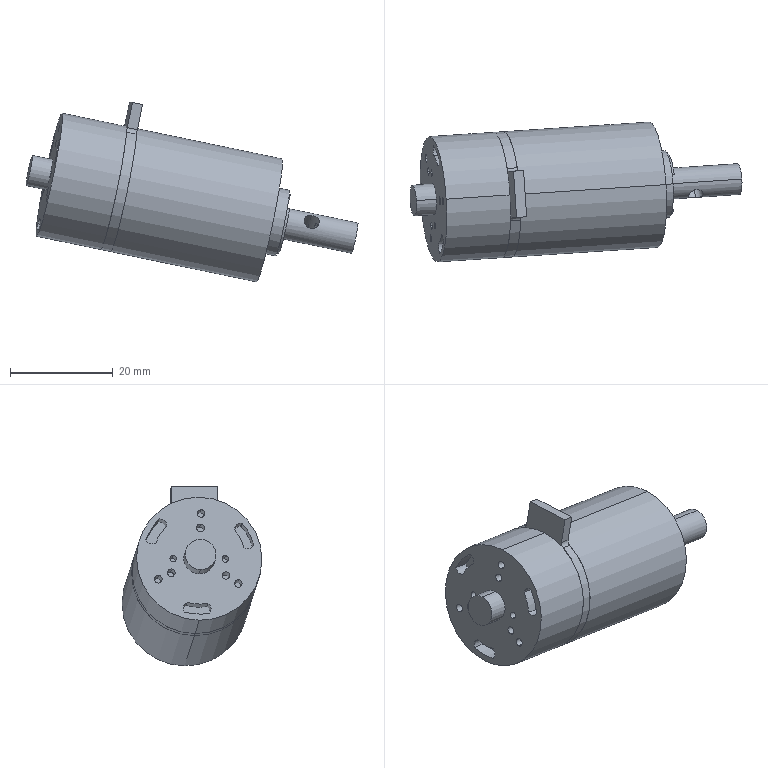Part | SolidWorks | features BaseBody 3 | 3 solids | 90 faces | box 64.493 x 27.178 x 34.913 mm | volume 21139 mm3 | cylinder 54 | plane 28 | cone 8 | commonest cylinder face diameters 1.5 x12 2.5 x8 2.828 x7 24.4 x6 1.3 x4 6 x4